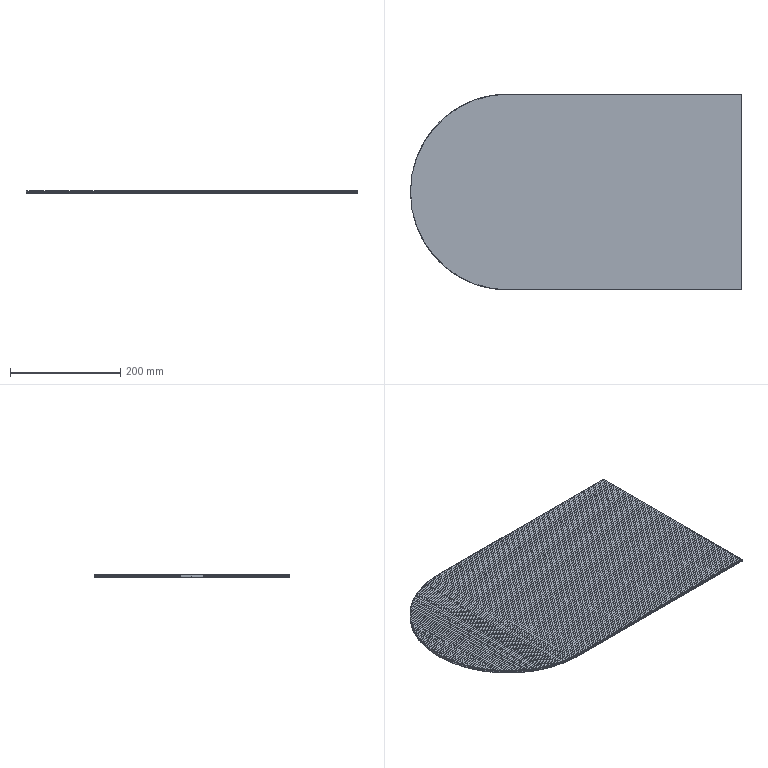Part | STEP file | 51E-01203JG10 | 1 solid | 323 faces | box 600 x 355 x 5 mm | volume 492755 mm3 | cylinder 317 | plane 6 | commonest cylinder face diameters 3.5 x315 355 x2